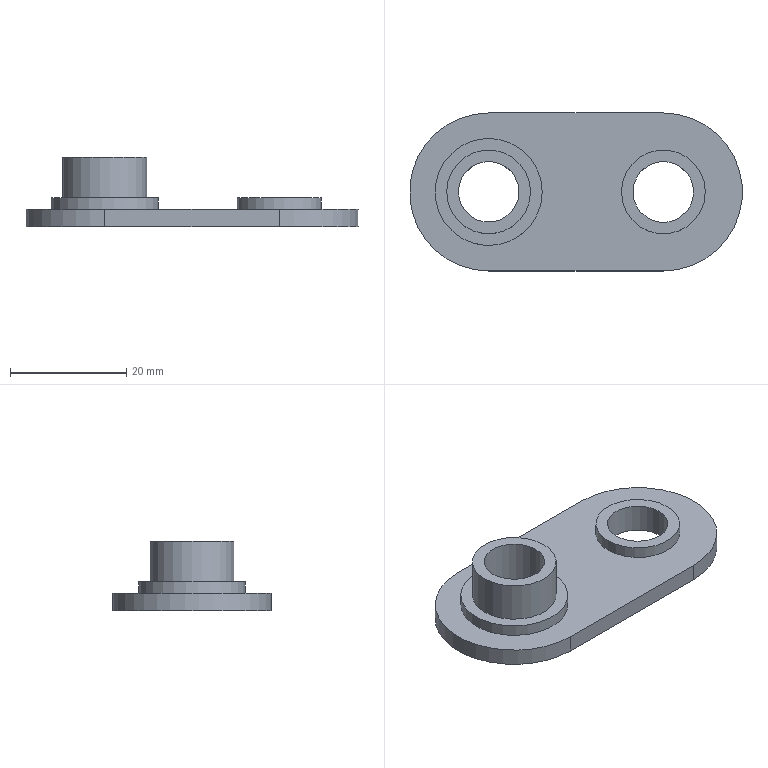Part | NX | features DATUM_CSYS 2, EXTRUDE 2, CYLINDER 1, REPLACE_FACE 1, SKETCH 1, UNITE 1 | 1 solid | 14 faces | box 57.14 x 27.14 x 12 mm | volume 4732 mm3 | plane 7 | cylinder 7 | commonest cylinder face diameters 10.4 x2 14.4 x2 27.14 x2 18.4 x1
STEP:
#1=CARTESIAN_POINT('',(7.2,-0.0005812,7.));
#2=VERTEX_POINT('',#1);
#3=CARTESIAN_POINT('',(-0.0004346,-0.0005812,7.));
#4=DIRECTION('',(0.,0.,-1.));
#5=DIRECTION('',(1.,0.,0.));
#6=AXIS2_PLACEMENT_3D('',#3,#4,#5);
#7=CIRCLE('',#6,7.2);
#8=EDGE_CURVE('',#2,#2,#7,.T.);
#9=ORIENTED_EDGE('',*,*,#8,.F.);
#10=EDGE_LOOP('',(#9));
#11=FACE_BOUND('',#10,.T.);
#12=CARTESIAN_POINT('',(5.2,-0.0005812,7.));
#13=VERTEX_POINT('',#12);
#14=CARTESIAN_POINT('',(-0.0004346,-0.0005812,7.));
#15=DIRECTION('',(0.,0.,1.));
#16=DIRECTION('',(1.,0.,0.));
#17=AXIS2_PLACEMENT_3D('',#14,#15,#16);
#18=CIRCLE('',#17,5.2);
#19=EDGE_CURVE('',#13,#13,#18,.F.);
#20=ORIENTED_EDGE('',*,*,#19,.T.);
#21=EDGE_LOOP('',(#20));
#22=FACE_BOUND('',#21,.T.);
#23=CARTESIAN_POINT('',(-0.0004346,-0.0005812,7.));
#24=DIRECTION('',(0.,0.,1.));
#25=DIRECTION('',(1.,0.,0.));
#26=AXIS2_PLACEMENT_3D('',#23,#24,#25);
#27=PLANE('',#26);
#28=ADVANCED_FACE('',(#11,#22),#27,.T.);
#29=CARTESIAN_POINT('',(-0.0004346,13.569,-5.));
#30=VERTEX_POINT('',#29);
#31=CARTESIAN_POINT('',(30.,13.569,-5.));
#32=VERTEX_POINT('',#31);
#33=CARTESIAN_POINT('',(-0.0004346,13.569,-5.));
#34=DIRECTION('',(1.,0.,0.));
#35=VECTOR('',#34,1000.);
#36=LINE('',#33,#35);
#37=EDGE_CURVE('',#30,#32,#36,.T.);
#38=ORIENTED_EDGE('',*,*,#37,.F.);
#39=CARTESIAN_POINT('',(-0.0004346,13.569,-2.));
#40=VERTEX_POINT('',#39);
#41=CARTESIAN_POINT('',(-0.0004346,13.569,-2.));
#42=DIRECTION('',(0.,0.,-1.));
#43=VECTOR('',#42,1000.);
#44=LINE('',#41,#43);
#45=EDGE_CURVE('',#40,#30,#44,.T.);
#46=ORIENTED_EDGE('',*,*,#45,.F.);
#47=CARTESIAN_POINT('',(30.,13.569,-2.));
#48=VERTEX_POINT('',#47);
#49=CARTESIAN_POINT('',(-0.0004346,13.569,-2.));
#50=DIRECTION('',(1.,0.,0.));
#51=VECTOR('',#50,1000.);
#52=LINE('',#49,#51);
#53=EDGE_CURVE('',#40,#48,#52,.T.);
#54=ORIENTED_EDGE('',*,*,#53,.T.);
#55=CARTESIAN_POINT('',(30.,13.569,-2.));
#56=DIRECTION('',(0.,0.,-1.));
#57=VECTOR('',#56,1000.);
#58=LINE('',#55,#57);
#59=EDGE_CURVE('',#48,#32,#58,.T.);
#60=ORIENTED_EDGE('',*,*,#59,.T.);
#61=EDGE_LOOP('',(#38,#46,#54,#60));
#62=FACE_BOUND('',#61,.T.);
#63=CARTESIAN_POINT('',(-0.0004346,13.569,-2.));
#64=DIRECTION('',(0.,1.,0.));
#65=DIRECTION('',(0.,0.,1.));
#66=AXIS2_PLACEMENT_3D('',#63,#64,#65);
#67=PLANE('',#66);
#68=ADVANCED_FACE('',(#62),#67,.T.);
#69=CARTESIAN_POINT('',(30.,-13.571,-5.));
#70=VERTEX_POINT('',#69);
#71=CARTESIAN_POINT('',(30.,-0.0005812,-5.));
#72=DIRECTION('',(0.,0.,-1.));
#73=DIRECTION('',(0.,-1.,0.));
#74=AXIS2_PLACEMENT_3D('',#71,#72,#73);
#75=CIRCLE('',#74,13.57);
#76=EDGE_CURVE('',#32,#70,#75,.T.);
#77=ORIENTED_EDGE('',*,*,#76,.F.);
#78=ORIENTED_EDGE('',*,*,#59,.F.);
#79=CARTESIAN_POINT('',(30.,-13.571,-2.));
#80=VERTEX_POINT('',#79);
#81=CARTESIAN_POINT('',(30.,-0.0005812,-2.));
#82=DIRECTION('',(0.,0.,-1.));
#83=DIRECTION('',(0.,-1.,0.));
#84=AXIS2_PLACEMENT_3D('',#81,#82,#83);
#85=CIRCLE('',#84,13.57);
#86=EDGE_CURVE('',#48,#80,#85,.T.);
#87=ORIENTED_EDGE('',*,*,#86,.T.);
#88=CARTESIAN_POINT('',(30.,-13.571,-2.));
#89=DIRECTION('',(0.,0.,-1.));
#90=VECTOR('',#89,1000.);
#91=LINE('',#88,#90);
#92=EDGE_CURVE('',#80,#70,#91,.T.);
#93=ORIENTED_EDGE('',*,*,#92,.T.);
#94=EDGE_LOOP('',(#77,#78,#87,#93));
#95=FACE_BOUND('',#94,.T.);
#96=CARTESIAN_POINT('',(30.,-0.0005812,-2.));
#97=DIRECTION('',(0.,0.,-1.));
#98=DIRECTION('',(-1.,0.,0.));
#99=AXIS2_PLACEMENT_3D('',#96,#97,#98);
#100=CYLINDRICAL_SURFACE('',#99,13.57);
#101=ADVANCED_FACE('',(#95),#100,.T.);
#102=CARTESIAN_POINT('',(-0.0004346,-13.571,-5.));
#103=VERTEX_POINT('',#102);
#104=CARTESIAN_POINT('',(30.,-13.571,-5.));
#105=DIRECTION('',(-1.,0.,0.));
#106=VECTOR('',#105,1000.);
#107=LINE('',#104,#106);
#108=EDGE_CURVE('',#70,#103,#107,.T.);
#109=ORIENTED_EDGE('',*,*,#108,.F.);
#110=ORIENTED_EDGE('',*,*,#92,.F.);
#111=CARTESIAN_POINT('',(-0.0004346,-13.571,-2.));
#112=VERTEX_POINT('',#111);
#113=CARTESIAN_POINT('',(30.,-13.571,-2.));
#114=DIRECTION('',(-1.,0.,0.));
#115=VECTOR('',#114,1000.);
#116=LINE('',#113,#115);
#117=EDGE_CURVE('',#80,#112,#116,.T.);
#118=ORIENTED_EDGE('',*,*,#117,.T.);
#119=CARTESIAN_POINT('',(-0.0004346,-13.571,-2.));
#120=DIRECTION('',(0.,0.,-1.));
#121=VECTOR('',#120,1000.);
#122=LINE('',#119,#121);
#123=EDGE_CURVE('',#112,#103,#122,.T.);
#124=ORIENTED_EDGE('',*,*,#123,.T.);
#125=EDGE_LOOP('',(#109,#110,#118,#124));
#126=FACE_BOUND('',#125,.T.);
#127=CARTESIAN_POINT('',(30.,-13.571,-2.));
#128=DIRECTION('',(0.,-1.,0.));
#129=DIRECTION('',(0.,0.,-1.));
#130=AXIS2_PLACEMENT_3D('',#127,#128,#129);
#131=PLANE('',#130);
#132=ADVANCED_FACE('',(#126),#131,.T.);
#133=ORIENTED_EDGE('',*,*,#19,.F.);
#134=EDGE_LOOP('',(#133));
#135=FACE_BOUND('',#134,.T.);
#136=CARTESIAN_POINT('',(5.2,-0.0005812,-5.));
#137=VERTEX_POINT('',#136);
#138=CARTESIAN_POINT('',(-0.0004346,-0.0005812,-5.));
#139=DIRECTION('',(0.,0.,-1.));
#140=DIRECTION('',(1.,0.,0.));
#141=AXIS2_PLACEMENT_3D('',#138,#139,#140);
#142=CIRCLE('',#141,5.2);
#143=EDGE_CURVE('',#137,#137,#142,.T.);
#144=ORIENTED_EDGE('',*,*,#143,.T.);
#145=EDGE_LOOP('',(#144));
#146=FACE_BOUND('',#145,.T.);
#147=CARTESIAN_POINT('',(-0.0004346,-0.0005812,-2.));
#148=DIRECTION('',(0.,0.,-1.));
#149=DIRECTION('',(-1.,0.,0.));
#150=AXIS2_PLACEMENT_3D('',#147,#148,#149);
#151=CYLINDRICAL_SURFACE('',#150,5.2);
#152=ADVANCED_FACE('',(#135,#146),#151,.F.);
#153=CARTESIAN_POINT('',(-0.0004346,-0.0005812,-5.));
#154=DIRECTION('',(0.,0.,-1.));
#155=DIRECTION('',(0.,1.,0.));
#156=AXIS2_PLACEMENT_3D('',#153,#154,#155);
#157=CIRCLE('',#156,13.57);
#158=EDGE_CURVE('',#103,#30,#157,.T.);
#159=ORIENTED_EDGE('',*,*,#158,.F.);
#160=ORIENTED_EDGE('',*,*,#123,.F.);
#161=CARTESIAN_POINT('',(-0.0004346,-0.0005812,-2.));
#162=DIRECTION('',(0.,0.,-1.));
#163=DIRECTION('',(0.,1.,0.));
#164=AXIS2_PLACEMENT_3D('',#161,#162,#163);
#165=CIRCLE('',#164,13.57);
#166=EDGE_CURVE('',#112,#40,#165,.T.);
#167=ORIENTED_EDGE('',*,*,#166,.T.);
#168=ORIENTED_EDGE('',*,*,#45,.T.);
#169=EDGE_LOOP('',(#159,#160,#167,#168));
#170=FACE_BOUND('',#169,.T.);
#171=CARTESIAN_POINT('',(-0.0004346,-0.0005812,-2.));
#172=DIRECTION('',(0.,0.,-1.));
#173=DIRECTION('',(-1.,0.,0.));
#174=AXIS2_PLACEMENT_3D('',#171,#172,#173);
#175=CYLINDRICAL_SURFACE('',#174,13.57);
#176=ADVANCED_FACE('',(#170),#175,.T.);
#177=CARTESIAN_POINT('',(35.2,-0.0005812,-5.));
#178=VERTEX_POINT('',#177);
#179=CARTESIAN_POINT('',(30.,-0.0005812,-5.));
#180=DIRECTION('',(0.,0.,-1.));
#181=DIRECTION('',(1.,0.,0.));
#182=AXIS2_PLACEMENT_3D('',#179,#180,#181);
#183=CIRCLE('',#182,5.2);
#184=EDGE_CURVE('',#178,#178,#183,.T.);
#185=ORIENTED_EDGE('',*,*,#184,.T.);
#186=EDGE_LOOP('',(#185));
#187=FACE_BOUND('',#186,.T.);
#188=CARTESIAN_POINT('',(35.2,-0.0005812,0.));
#189=VERTEX_POINT('',#188);
#190=CARTESIAN_POINT('',(30.,-0.0005812,0.));
#191=DIRECTION('',(0.,0.,-1.));
#192=DIRECTION('',(1.,0.,0.));
#193=AXIS2_PLACEMENT_3D('',#190,#191,#192);
#194=CIRCLE('',#193,5.2);
#195=EDGE_CURVE('',#189,#189,#194,.T.);
#196=ORIENTED_EDGE('',*,*,#195,.F.);
#197=EDGE_LOOP('',(#196));
#198=FACE_BOUND('',#197,.T.);
#199=CARTESIAN_POINT('',(30.,-0.0005812,-2.));
#200=DIRECTION('',(0.,0.,-1.));
#201=DIRECTION('',(-1.,0.,0.));
#202=AXIS2_PLACEMENT_3D('',#199,#200,#201);
#203=CYLINDRICAL_SURFACE('',#202,5.2);
#204=ADVANCED_FACE('',(#187,#198),#203,.F.);
#205=CARTESIAN_POINT('',(37.2,-0.0005812,-2.));
#206=VERTEX_POINT('',#205);
#207=CARTESIAN_POINT('',(30.,-0.0005812,-2.));
#208=DIRECTION('',(0.,0.,1.));
#209=DIRECTION('',(1.,0.,0.));
#210=AXIS2_PLACEMENT_3D('',#207,#208,#209);
#211=CIRCLE('',#210,7.2);
#212=EDGE_CURVE('',#206,#206,#211,.T.);
#213=ORIENTED_EDGE('',*,*,#212,.F.);
#214=EDGE_LOOP('',(#213));
#215=FACE_BOUND('',#214,.T.);
#216=CARTESIAN_POINT('',(9.2,-0.0005812,-2.));
#217=VERTEX_POINT('',#216);
#218=CARTESIAN_POINT('',(-0.0004346,-0.0005812,-2.));
#219=DIRECTION('',(0.,0.,1.));
#220=DIRECTION('',(1.,0.,0.));
#221=AXIS2_PLACEMENT_3D('',#218,#219,#220);
#222=CIRCLE('',#221,9.2);
#223=EDGE_CURVE('',#217,#217,#222,.T.);
#224=ORIENTED_EDGE('',*,*,#223,.F.);
#225=EDGE_LOOP('',(#224));
#226=FACE_BOUND('',#225,.T.);
#227=ORIENTED_EDGE('',*,*,#53,.F.);
#228=ORIENTED_EDGE('',*,*,#166,.F.);
#229=ORIENTED_EDGE('',*,*,#117,.F.);
#230=ORIENTED_EDGE('',*,*,#86,.F.);
#231=EDGE_LOOP('',(#227,#228,#229,#230));
#232=FACE_BOUND('',#231,.T.);
#233=CARTESIAN_POINT('',(30.,-0.0005812,-2.));
#234=DIRECTION('',(0.,0.,-1.));
#235=DIRECTION('',(-1.,0.,0.));
#236=AXIS2_PLACEMENT_3D('',#233,#234,#235);
#237=PLANE('',#236);
#238=ADVANCED_FACE('',(#215,#226,#232),#237,.F.);
#239=ORIENTED_EDGE('',*,*,#37,.T.);
#240=ORIENTED_EDGE('',*,*,#76,.T.);
#241=ORIENTED_EDGE('',*,*,#108,.T.);
#242=ORIENTED_EDGE('',*,*,#158,.T.);
#243=EDGE_LOOP('',(#239,#240,#241,#242));
#244=FACE_BOUND('',#243,.T.);
#245=ORIENTED_EDGE('',*,*,#143,.F.);
#246=EDGE_LOOP('',(#245));
#247=FACE_BOUND('',#246,.T.);
#248=ORIENTED_EDGE('',*,*,#184,.F.);
#249=EDGE_LOOP('',(#248));
#250=FACE_BOUND('',#249,.T.);
#251=CARTESIAN_POINT('',(30.,-0.0005812,-5.));
#252=DIRECTION('',(0.,0.,-1.));
#253=DIRECTION('',(-1.,0.,0.));
#254=AXIS2_PLACEMENT_3D('',#251,#252,#253);
#255=PLANE('',#254);
#256=ADVANCED_FACE('',(#244,#247,#250),#255,.T.);
#257=CARTESIAN_POINT('',(7.2,-0.0005812,0.));
#258=VERTEX_POINT('',#257);
#259=CARTESIAN_POINT('',(-0.0004346,-0.0005812,0.));
#260=DIRECTION('',(0.,0.,1.));
#261=DIRECTION('',(1.,0.,0.));
#262=AXIS2_PLACEMENT_3D('',#259,#260,#261);
#263=CIRCLE('',#262,7.2);
#264=EDGE_CURVE('',#258,#258,#263,.T.);
#265=ORIENTED_EDGE('',*,*,#264,.T.);
#266=EDGE_LOOP('',(#265));
#267=FACE_BOUND('',#266,.T.);
#268=ORIENTED_EDGE('',*,*,#8,.T.);
#269=EDGE_LOOP('',(#268));
#270=FACE_BOUND('',#269,.T.);
#271=CARTESIAN_POINT('',(-0.0004346,-0.0005812,-2.));
#272=DIRECTION('',(0.,0.,1.));
#273=DIRECTION('',(1.,0.,0.));
#274=AXIS2_PLACEMENT_3D('',#271,#272,#273);
#275=CYLINDRICAL_SURFACE('',#274,7.2);
#276=ADVANCED_FACE('',(#267,#270),#275,.T.);
#277=ORIENTED_EDGE('',*,*,#264,.F.);
#278=EDGE_LOOP('',(#277));
#279=FACE_BOUND('',#278,.T.);
#280=CARTESIAN_POINT('',(9.2,-0.0005812,0.));
#281=VERTEX_POINT('',#280);
#282=CARTESIAN_POINT('',(-0.0004346,-0.0005812,0.));
#283=DIRECTION('',(0.,0.,1.));
#284=DIRECTION('',(1.,0.,0.));
#285=AXIS2_PLACEMENT_3D('',#282,#283,#284);
#286=CIRCLE('',#285,9.2);
#287=EDGE_CURVE('',#281,#281,#286,.T.);
#288=ORIENTED_EDGE('',*,*,#287,.T.);
#289=EDGE_LOOP('',(#288));
#290=FACE_BOUND('',#289,.T.);
#291=CARTESIAN_POINT('',(-0.0004346,-0.0005812,0.));
#292=DIRECTION('',(0.,0.,1.));
#293=DIRECTION('',(1.,0.,0.));
#294=AXIS2_PLACEMENT_3D('',#291,#292,#293);
#295=PLANE('',#294);
#296=ADVANCED_FACE('',(#279,#290),#295,.T.);
#297=ORIENTED_EDGE('',*,*,#223,.T.);
#298=EDGE_LOOP('',(#297));
#299=FACE_BOUND('',#298,.T.);
#300=ORIENTED_EDGE('',*,*,#287,.F.);
#301=EDGE_LOOP('',(#300));
#302=FACE_BOUND('',#301,.T.);
#303=CARTESIAN_POINT('',(-0.0004346,-0.0005812,-2.));
#304=DIRECTION('',(0.,0.,1.));
#305=DIRECTION('',(1.,0.,0.));
#306=AXIS2_PLACEMENT_3D('',#303,#304,#305);
#307=CYLINDRICAL_SURFACE('',#306,9.2);
#308=ADVANCED_FACE('',(#299,#302),#307,.T.);
#309=ORIENTED_EDGE('',*,*,#212,.T.);
#310=EDGE_LOOP('',(#309));
#311=FACE_BOUND('',#310,.T.);
#312=CARTESIAN_POINT('',(37.2,-0.0005812,0.));
#313=VERTEX_POINT('',#312);
#314=CARTESIAN_POINT('',(30.,-0.0005812,0.));
#315=DIRECTION('',(0.,0.,1.));
#316=DIRECTION('',(1.,0.,0.));
#317=AXIS2_PLACEMENT_3D('',#314,#315,#316);
#318=CIRCLE('',#317,7.2);
#319=EDGE_CURVE('',#313,#313,#318,.T.);
#320=ORIENTED_EDGE('',*,*,#319,.F.);
#321=EDGE_LOOP('',(#320));
#322=FACE_BOUND('',#321,.T.);
#323=CARTESIAN_POINT('',(30.,-0.0005812,-2.));
#324=DIRECTION('',(0.,0.,1.));
#325=DIRECTION('',(1.,0.,0.));
#326=AXIS2_PLACEMENT_3D('',#323,#324,#325);
#327=CYLINDRICAL_SURFACE('',#326,7.2);
#328=ADVANCED_FACE('',(#311,#322),#327,.T.);
#329=ORIENTED_EDGE('',*,*,#319,.T.);
#330=EDGE_LOOP('',(#329));
#331=FACE_BOUND('',#330,.T.);
#332=ORIENTED_EDGE('',*,*,#195,.T.);
#333=EDGE_LOOP('',(#332));
#334=FACE_BOUND('',#333,.T.);
#335=CARTESIAN_POINT('',(30.,-0.0005812,0.));
#336=DIRECTION('',(0.,0.,1.));
#337=DIRECTION('',(1.,0.,0.));
#338=AXIS2_PLACEMENT_3D('',#335,#336,#337);
#339=PLANE('',#338);
#340=ADVANCED_FACE('',(#331,#334),#339,.T.);
#341=CLOSED_SHELL('',(#28,#68,#101,#132,#152,#176,#204,#238,#256,#276,#296,#308,#328,#340));
#342=MANIFOLD_SOLID_BREP('',#341);
#343=(LENGTH_UNIT()NAMED_UNIT(*)SI_UNIT(.MILLI.,.METRE.));
#344=UNCERTAINTY_MEASURE_WITH_UNIT(LENGTH_MEASURE(0.00001),#343,'','');
#345=(NAMED_UNIT(*)PLANE_ANGLE_UNIT()SI_UNIT($,.RADIAN.));
#346=(NAMED_UNIT(*)SI_UNIT($,.STERADIAN.)SOLID_ANGLE_UNIT());
#347=(GEOMETRIC_REPRESENTATION_CONTEXT(3)GLOBAL_UNCERTAINTY_ASSIGNED_CONTEXT((#344))GLOBAL_UNIT_ASSIGNED_CONTEXT((#343,#345,#346))REPRESENTATION_CONTEXT('',''));
#348=ADVANCED_BREP_SHAPE_REPRESENTATION('',(#342),#347);